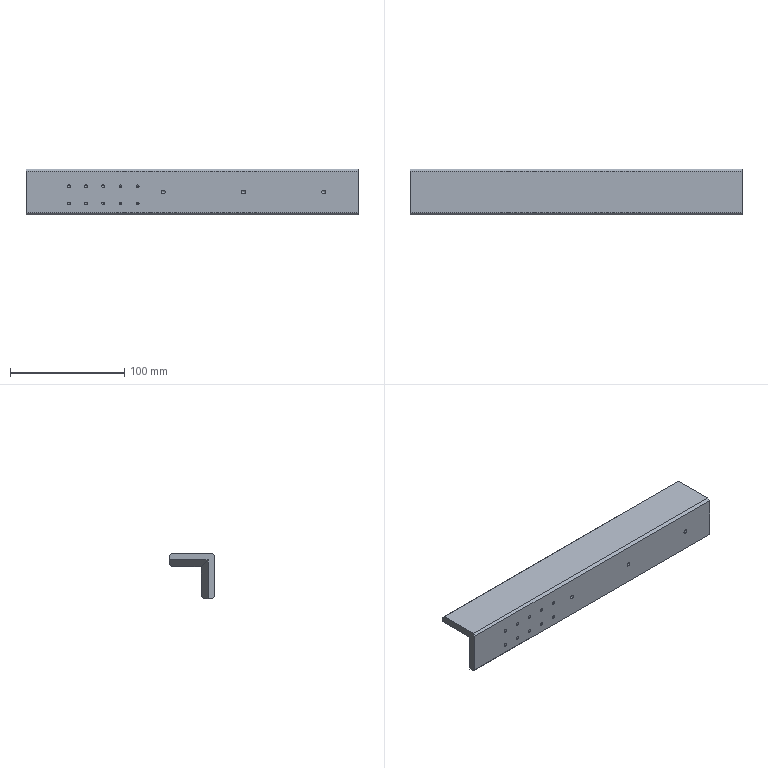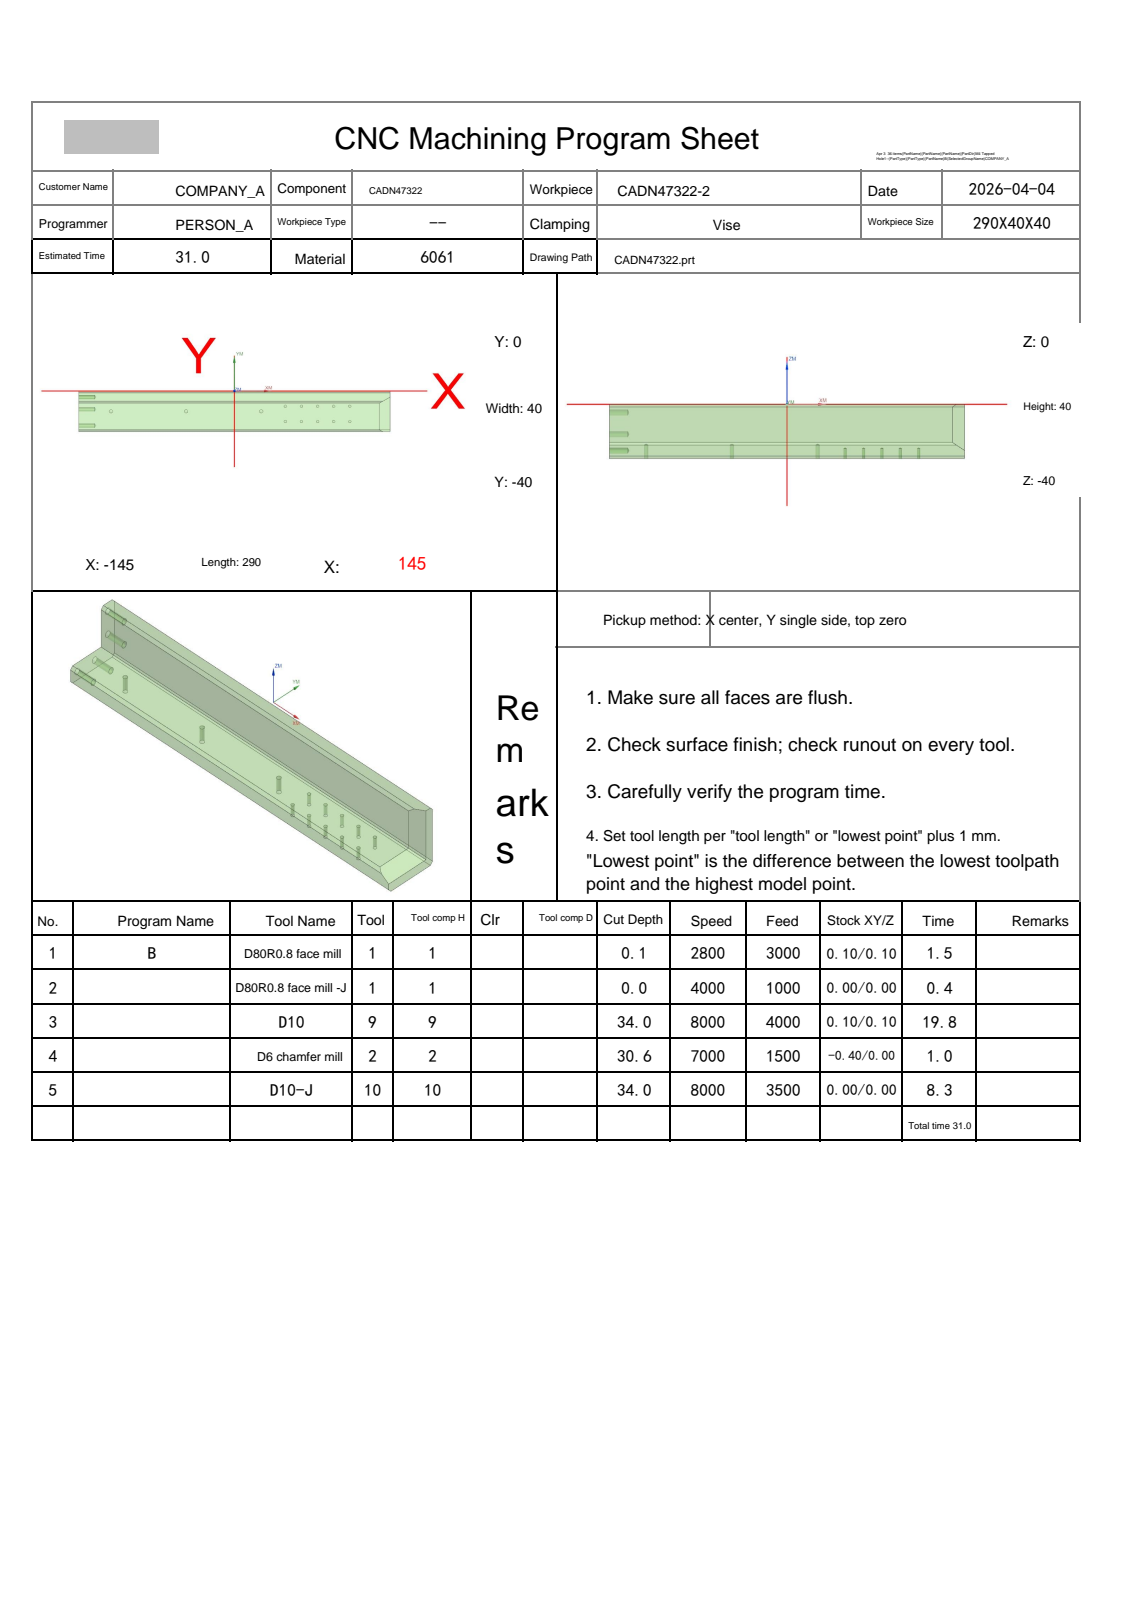NC program | NX | posted by the shop | part box 290 x 40 x 40 mm
Lines 3474 to 6219 of 6219, first 2289 of 2746 lines:
N4 T02 M06
(D6 chamfer mill  D=6. R=0. H=02 ce=0.00 di=0.00)
G00 G90 G54 X145.99 Y-1.208 M03 S6500
G43 H02 Z20.
M08
Z.13
G01 Z-1.2 F1500.
G03 X145.915 Y-1.548 I1.907 J-.601
G01 X145.905 Y-1.602
X145.928 Y-1.651
X145.966 Y-1.741
X146. Y-2.
Y-6.
X145.967 Y-6.255
X145.87 Y-6.493
X145.716 Y-6.698
X145.514 Y-6.857
X138.848 Y-10.857
X138.6 Y-10.964
X138.534 Y-10.973
X138.51 Y-10.969
X138.495 Y-10.989
X138.435 Y-11.027
X138.393 Y-11.083
Z.314
G00 Z10.
X-145.99 Y-10.792
Z.13
G01 Z-1.2
G03 X-145.915 Y-10.452 I-1.907 J.601
G01 X-145.905 Y-10.398
X-145.928 Y-10.349
X-145.966 Y-10.259
X-146. Y-10.
Y-2.
X-145.966 Y-1.741
X-145.928 Y-1.651
X-145.905 Y-1.602
X-145.915 Y-1.548
G03 X-145.99 Y-1.208 I-1.983 J-.261
G01 Z.13
G00 Z10.
X-145.916 Y-38.379
Z-25.199
G01 Z-29.199
X-145.966 Y-38.259
X-146. Y-38.
Y-15.123
X-146.008 Y-15.093
X-146.068 Y-15.007
Z-3.084
G00 Z20.
G00 G90 X-148.9 Y1.516 M03 S6500
Z20.
Z-1.2
G01 Z-2.7 F1000.
G03 X-147.763 Y.7 I1.137 J.384
G01 X147.763
G03 X148.9 Y1.516 I0.0 J1.2
G01 Z-1.2
G00 Z20.
X140.284 Y-13.378
Z-1.2
G01 Z-2.7
G03 X139.204 Y-12.7 I-1.08 J-.522
G01 X-147.763
G03 X-148.9 Y-13.516 I0.0 J-1.2
G01 Z-1.2
G00 Z20.
G00 G90 X142.5 Y-40.6 M03 S7000
Z20.
Z-28.1
G01 Z-30.6 F1000.
X135.
X-145.
X-152.5
Z-28.1
G00 Z20.
G91 G28 Z0.0
M05
M09
G91 G28 Z0.0
M01
N5 T10 M06
(D10-J  D=10. R=0. H=10 ce=0.40 di=0.00)
G00 G90 G54 X142. Y-40.999 M03 S7000
G43 H10 Z14.5
M08
Z-26.5
G01 Z-28. F1500.
G03 X140. Y-39. I-2. J-.001
G01 X-149.1
G02 X-150. Y-38.1 I0.0 J.9
G01 Y-35.68
G02 X-149. Y-34.68 I1. J0.0
G01 X139.1
G03 X140. Y-33.78 I0.0 J.9
G01 Y-31.36
G03 X139. Y-30.36 I-1. J0.0
G01 X-149.1
G02 X-150. Y-29.46 I0.0 J.9
G01 Y-27.04
G02 X-149. Y-26.04 I1. J0.0
G01 X139.1
G03 X140. Y-25.14 I0.0 J.9
G01 Y-22.72
G03 X139. Y-21.72 I-1. J0.0
G01 X-149.1
G02 X-150. Y-20.82 I0.0 J.9
G01 Y-18.4
G02 X-149. Y-17.4 I1. J0.0
G01 X140.
G02 X142. Y-19.399 I0.0 J-2.
G01 Z-26.5
G00 Z14.5
G00 G90 X149.655 Y-10.817 M03 S8000
Z9.5
Z-13.
G01 Z-14. F1000.
G41 D10
X149.533 Y-10.659
G03 X148.344 Y-10.074 I-1.189 J-.915
X147.572 Y-10.287 I0.0 J-1.5
G01 X137.572 Y-16.287
G02 X135. Y-17. I-2.572 J4.287
G01 X-145.
G03 X-146.49 Y-18.327 I0.0 J-1.5
G01 G40 X-146.513 Y-18.526
Z-13.
G00 Z9.5
X149.655 Y-10.817
Z-27.
G01 Z-28.
G41 D10
X149.533 Y-10.659
G03 X148.344 Y-10.074 I-1.189 J-.915
X147.572 Y-10.287 I0.0 J-1.5
G01 X137.572 Y-16.287
G02 X135. Y-17. I-2.572 J4.287
G01 X-145.
G03 X-146.49 Y-18.327 I0.0 J-1.5
G01 G40 X-146.513 Y-18.526
Z-27.
G00 Z9.5
G00 G90 X145.023 Y-17.66 M03 S7000
Z14.5
Z-27.508
G01 Z-28.008 F3500.
X140.023 Y-14.829
Y-39.163
X140.021 Y-39.21
X140.034 Y-39.218 Z-28.015
X140.036 Y-39.163
Y-14.821
X140.049 Y-14.813 Z-28.023
Y-39.163
X140.046 Y-39.226
X140.059 Y-39.233 Z-28.031
X140.061 Y-39.163
Y-14.806
X140.074 Y-14.798 Z-28.039
Y-39.163
X140.072 Y-39.241
X140.084 Y-39.249 Z-28.046
X140.087 Y-39.163
Y-14.79
X140.1 Y-14.783 Z-28.054
Y-39.163
X140.097 Y-39.257
X140.11 Y-39.265 Z-28.062
X140.113 Y-39.163
Y-14.775
X140.126 Y-14.767 Z-28.069
Y-39.163
X140.123 Y-39.272
X140.135 Y-39.28 Z-28.077
X140.139 Y-39.163
Y-14.759
X140.151 Y-14.752 Z-28.085
Y-39.163
X140.148 Y-39.288
X140.161 Y-39.296 Z-28.093
X140.164 Y-39.163
Y-14.744
X140.177 Y-14.736 Z-28.1
Y-39.163
X140.174 Y-39.304
X140.187 Y-39.311 Z-28.108
X140.19 Y-39.163
Y-14.729
X140.203 Y-14.721 Z-28.116
Y-39.163
X140.2 Y-39.319
X140.213 Y-39.327 Z-28.123
X140.216 Y-39.163
Y-14.713
X140.229 Y-14.705 Z-28.131
Y-39.163
X140.226 Y-39.335
X140.238 Y-39.343 Z-28.139
X140.242 Y-39.163
Y-14.698
X140.254 Y-14.69 Z-28.147
Y-39.163
X140.251 Y-39.35
X140.266 Y-39.358 Z-28.154
X140.267 Y-39.163
Y-14.682
X140.28 Y-14.675 Z-28.162
Y-39.163
X140.277 Y-39.366
X140.29 Y-39.374 Z-28.17
X140.293 Y-39.163
Y-14.667
X140.306 Y-14.659 Z-28.178
Y-39.163
X140.303 Y-39.382
X140.316 Y-39.389 Z-28.185
X140.319 Y-39.163
Y-14.651
X140.332 Y-14.644 Z-28.193
Y-39.163
X140.329 Y-39.397
X140.342 Y-39.405 Z-28.201
X140.344 Y-38.201
Y-14.636
X140.357 Y-14.628 Z-28.208
Y-38.208
X140.355 Y-39.413
X140.367 Y-39.421 Z-28.216
X140.37 Y-38.216
Y-14.621
X140.383 Y-14.613 Z-28.224
Y-38.224
X140.38 Y-39.428
X140.393 Y-39.436 Z-28.232
X140.396 Y-38.232
Y-14.605
X140.409 Y-14.597 Z-28.239
Y-38.239
X140.406 Y-39.444
X140.419 Y-39.452 Z-28.247
X140.422 Y-38.247
Y-14.59
X140.434 Y-14.582 Z-28.255
Y-38.255
X140.432 Y-39.459
X140.445 Y-39.467 Z-28.262
X140.447 Y-38.262
Y-14.574
X140.46 Y-14.567 Z-28.27
Y-38.27
X140.458 Y-39.475
X140.471 Y-39.483 Z-28.278
X140.473 Y-38.278
Y-14.559
X140.486 Y-14.551 Z-28.286
Y-38.286
X140.484 Y-39.491
X140.497 Y-39.498 Z-28.293
X140.499 Y-38.293
Y-14.543
X140.512 Y-14.536 Z-28.301
Y-38.301
X140.51 Y-39.506
X140.523 Y-39.514 Z-28.309
X140.524 Y-38.309
Y-14.528
X140.537 Y-14.52 Z-28.316
Y-38.316
X140.536 Y-39.522
X140.549 Y-39.53 Z-28.324
X140.55 Y-38.324
Y-14.512
X140.563 Y-14.505 Z-28.332
Y-38.332
X140.562 Y-39.537
X140.575 Y-39.545 Z-28.34
X140.576 Y-38.34
Y-14.497
X140.589 Y-14.489 Z-28.347
Y-38.347
X140.588 Y-39.553
X140.601 Y-39.561 Z-28.355
X140.602 Y-38.355
Y-14.482
X140.615 Y-14.474 Z-28.363
Y-38.363
X140.614 Y-39.569
X140.627 Y-39.576 Z-28.37
Y-38.37
Y-14.466
X140.64 Y-14.458 Z-28.378
Y-38.378
Y-39.584
X140.653 Y-39.592 Z-28.386
Y-38.386
Y-14.451
X140.666 Y-14.443 Z-28.394
Y-38.394
Y-39.6
X140.679 Y-39.607 Z-28.401
Y-38.401
Y-14.435
X140.692 Y-14.428 Z-28.409
Y-38.409
X140.691 Y-39.615
X140.704 Y-39.623 Z-28.417
X140.705 Y-38.417
Y-14.42
X140.717 Y-14.412 Z-28.424
Y-38.424
Y-39.631
X140.729 Y-39.638 Z-28.432
X140.73 Y-39.61
Y-14.404
X140.743 Y-14.397 Z-28.44
Y-39.61
X140.742 Y-39.646
X140.754 Y-39.654 Z-28.448
X140.756 Y-39.61
Y-14.389
X140.769 Y-14.381 Z-28.455
Y-39.61
X140.767 Y-39.661
X140.78 Y-39.669 Z-28.463
X140.782 Y-39.61
Y-14.374
X140.795 Y-14.366 Z-28.471
Y-39.61
X140.792 Y-39.677
X140.805 Y-39.685 Z-28.478
X140.807 Y-39.61
Y-14.358
X140.82 Y-14.35 Z-28.486
Y-39.61
X140.818 Y-39.692
X140.83 Y-39.7 Z-28.494
X140.833 Y-39.61
Y-14.343
X140.846 Y-14.335 Z-28.502
Y-39.61
X140.843 Y-39.708
X140.856 Y-39.715 Z-28.509
X140.859 Y-39.61
Y-14.327
X140.872 Y-14.32 Z-28.517
Y-39.61
X140.869 Y-39.723
X140.881 Y-39.731 Z-28.525
X140.885 Y-39.61
Y-14.312
X140.898 Y-14.304 Z-28.533
Y-39.61
X140.894 Y-39.738
X140.907 Y-39.746 Z-28.54
X140.91 Y-39.61
Y-14.296
X140.923 Y-14.289 Z-28.548
Y-39.61
X140.92 Y-39.754
X140.933 Y-39.761 Z-28.556
X140.936 Y-39.61
Y-14.281
X140.949 Y-14.273 Z-28.563
Y-39.61
X140.945 Y-39.769
X140.958 Y-39.777 Z-28.571
X140.962 Y-39.61
Y-14.266
X140.975 Y-14.258 Z-28.579
Y-39.61
X140.971 Y-39.785
X140.984 Y-39.792 Z-28.587
X140.988 Y-39.61
Y-14.25
X141. Y-14.242 Z-28.594
Y-39.61
X140.997 Y-39.8
X141.01 Y-39.808 Z-28.602
X141.013 Y-39.61
Y-14.235
X141.026 Y-14.227 Z-28.61
Y-39.61
X141.023 Y-39.815
X141.036 Y-39.823 Z-28.617
X141.039 Y-39.61
Y-14.219
X141.052 Y-14.212 Z-28.625
Y-39.61
X141.049 Y-39.831
X141.062 Y-39.838 Z-28.633
X141.065 Y-39.61
Y-14.204
X141.078 Y-14.196 Z-28.641
Y-39.61
X141.075 Y-39.846
X141.088 Y-39.854 Z-28.648
X141.09 Y-38.648
Y-14.188
X141.103 Y-14.181 Z-28.656
Y-38.656
X141.101 Y-39.862
X141.114 Y-39.869 Z-28.664
X141.116 Y-38.664
Y-14.173
X141.129 Y-14.165 Z-28.671
Y-38.671
X141.127 Y-39.877
X141.14 Y-39.885 Z-28.679
X141.142 Y-38.679
Y-14.157
X141.155 Y-14.15 Z-28.687
Y-38.687
X141.153 Y-39.892
X141.166 Y-39.9 Z-28.695
X141.168 Y-38.695
Y-14.142
X141.18 Y-14.134 Z-28.702
Y-38.702
X141.179 Y-39.908
X141.192 Y-39.915 Z-28.71
X141.193 Y-38.71
Y-14.127
X141.206 Y-14.119 Z-28.718
Y-38.718
X141.205 Y-39.923
X141.218 Y-39.931 Z-28.725
X141.219 Y-38.725
Y-14.111
X141.232 Y-14.103 Z-28.733
Y-38.733
X141.23 Y-39.939
X141.243 Y-39.946 Z-28.741
X141.245 Y-38.741
Y-14.096
X141.258 Y-14.088 Z-28.749
Y-38.749
X141.256 Y-39.954
X141.269 Y-39.962 Z-28.756
X141.271 Y-38.756
Y-14.08
X141.283 Y-14.073 Z-28.764
Y-38.764
X141.282 Y-39.969
X141.295 Y-39.977 Z-28.772
X141.296 Y-38.772
Y-14.065
X141.309 Y-14.057 Z-28.779
Y-38.779
X141.308 Y-39.985
X141.321 Y-39.992 Z-28.787
X141.322 Y-38.787
Y-14.049
X141.335 Y-14.042 Z-28.795
Y-38.795
X141.334 Y-40.
X141.347 Y-40.008 Z-28.803
X141.348 Y-38.803
Y-14.034
X141.361 Y-14.026 Z-28.81
Y-38.81
X141.36 Y-40.016
X141.373 Y-40.023 Z-28.818
Y-38.818
Y-14.019
X141.386 Y-14.011 Z-28.826
Y-38.826
Y-40.031
X141.399 Y-40.039 Z-28.833
Y-38.834
Y-14.003
X141.412 Y-13.995 Z-28.841
Y-38.841
Y-40.046
X141.425 Y-40.054 Z-28.849
Y-38.849
Y-13.988
X141.438 Y-13.98 Z-28.857
Y-38.857
Y-40.062
X141.45 Y-40.069 Z-28.864
X141.451 Y-38.864
Y-13.972
X141.463 Y-13.965 Z-28.872
Y-38.872
Y-40.077
X141.475 Y-40.085 Z-28.88
X141.476 Y-40.057
Y-13.957
X141.489 Y-13.949 Z-28.888
Y-40.057
X141.488 Y-40.092
X141.5 Y-40.1 Z-28.895
X141.502 Y-40.057
Y-13.941
X141.515 Y-13.934 Z-28.903
Y-40.057
X141.513 Y-40.108
X141.526 Y-40.116 Z-28.911
X141.528 Y-40.057
Y-13.926
X141.541 Y-13.918 Z-28.918
Y-40.057
X141.538 Y-40.123
X141.551 Y-40.131 Z-28.926
X141.553 Y-40.057
Y-13.911
X141.566 Y-13.903 Z-28.934
Y-40.057
X141.564 Y-40.139
X141.577 Y-40.146 Z-28.942
X141.579 Y-40.057
Y-13.895
X141.592 Y-13.887 Z-28.949
Y-40.057
X141.589 Y-40.154
X141.602 Y-40.162 Z-28.957
X141.605 Y-40.057
Y-13.88
X141.618 Y-13.872 Z-28.965
Y-40.057
X141.615 Y-40.169
X141.628 Y-40.177 Z-28.972
X141.631 Y-40.057
Y-13.864
X141.644 Y-13.857 Z-28.98
Y-40.057
X141.64 Y-40.185
X141.653 Y-40.192 Z-28.988
X141.656 Y-40.057
Y-13.849
X141.669 Y-13.841 Z-28.996
Y-40.057
X141.666 Y-40.2
X141.679 Y-40.208 Z-29.003
X141.682 Y-40.057
Y-13.833
X141.695 Y-13.826 Z-29.011
Y-40.057
X141.692 Y-40.215
X141.704 Y-40.223 Z-29.019
X141.708 Y-40.057
Y-13.818
X141.721 Y-13.81 Z-29.026
Y-40.057
X141.717 Y-40.231
X141.73 Y-40.238 Z-29.034
X141.734 Y-40.057
Y-13.802
X141.746 Y-13.795 Z-29.042
Y-40.057
X141.743 Y-40.246
X141.756 Y-40.253 Z-29.05
X141.759 Y-40.057
Y-13.787
X141.772 Y-13.779 Z-29.057
Y-40.057
X141.769 Y-40.261
X141.782 Y-40.269 Z-29.065
X141.785 Y-40.057
Y-13.772
X141.798 Y-13.764 Z-29.073
Y-40.057
X141.795 Y-40.276
X141.807 Y-40.284 Z-29.08
X141.811 Y-40.057
Y-13.756
X141.824 Y-13.748 Z-29.088
Y-40.057
X141.82 Y-40.292
X141.833 Y-40.299 Z-29.096
X141.836 Y-39.096
Y-13.741
X141.849 Y-13.733 Z-29.104
Y-39.104
X141.846 Y-40.307
X141.859 Y-40.315 Z-29.111
X141.862 Y-39.111
Y-13.725
X141.875 Y-13.718 Z-29.119
Y-39.119
X141.872 Y-40.322
X141.885 Y-40.33 Z-29.127
X141.888 Y-39.127
Y-13.71
X141.901 Y-13.702 Z-29.134
Y-39.134
X141.898 Y-40.338
X141.911 Y-40.345 Z-29.142
X141.914 Y-39.142
Y-13.694
X141.926 Y-13.687 Z-29.15
Y-39.15
X141.924 Y-40.353
X141.937 Y-40.361 Z-29.158
X141.939 Y-39.158
Y-13.679
X141.952 Y-13.671 Z-29.165
Y-39.165
X141.95 Y-40.368
X141.963 Y-40.376 Z-29.173
X141.965 Y-39.173
Y-13.664
X141.978 Y-13.656 Z-29.181
Y-39.181
X141.976 Y-40.384
X141.989 Y-40.391 Z-29.188
X141.991 Y-39.189
Y-13.648
X142.004 Y-13.64 Z-29.196
Y-39.196
X142.002 Y-40.399
X142.016 Y-40.407 Z-29.204
X142.017 Y-39.204
Y-13.633
X142.029 Y-13.625 Z-29.212
Y-39.212
Y-40.414
X142.042 Y-40.422 Z-29.219
Y-39.219
Y-13.617
X142.055 Y-13.61 Z-29.227
Y-39.227
Y-40.429
X142.067 Y-40.437 Z-29.235
X142.068 Y-39.235
Y-13.602
X142.081 Y-13.594 Z-29.243
Y-39.243
X142.08 Y-40.445
X142.093 Y-40.452 Z-29.25
X142.094 Y-39.25
Y-13.586
X142.107 Y-13.579 Z-29.258
Y-39.258
X142.106 Y-40.46
X142.119 Y-40.467 Z-29.266
Y-39.266
Y-13.571
X142.132 Y-13.563 Z-29.273
Y-39.273
Y-40.475
X142.145 Y-40.483 Z-29.281
Y-39.281
Y-13.556
X142.158 Y-13.548 Z-29.289
Y-39.289
Y-40.49
X142.171 Y-40.498 Z-29.297
Y-39.297
Y-13.54
X142.184 Y-13.532 Z-29.304
Y-39.304
Y-40.505
X142.196 Y-40.513 Z-29.312
X142.197 Y-39.312
Y-13.525
X142.209 Y-13.517 Z-29.32
Y-39.32
Y-40.521
X142.221 Y-40.528 Z-29.327
X142.222 Y-39.327
Y-13.509
X142.235 Y-13.501 Z-29.335
Y-40.505
X142.234 Y-40.536
X142.246 Y-40.543 Z-29.343
X142.248 Y-40.505
Y-13.494
X142.261 Y-13.486 Z-29.351
Y-40.505
X142.259 Y-40.551
X142.272 Y-40.558 Z-29.358
X142.274 Y-40.505
Y-13.478
X142.287 Y-13.471 Z-29.366
Y-40.505
X142.284 Y-40.566
X142.297 Y-40.574 Z-29.374
X142.3 Y-40.505
Y-13.463
X142.312 Y-13.455 Z-29.381
Y-40.505
X142.31 Y-40.581
X142.322 Y-40.589 Z-29.389
X142.325 Y-40.505
Y-13.447
X142.338 Y-13.44 Z-29.397
Y-40.505
X142.335 Y-40.596
X142.348 Y-40.604 Z-29.405
X142.351 Y-40.505
Y-13.432
X142.364 Y-13.424 Z-29.412
Y-40.505
X142.361 Y-40.612
X142.374 Y-40.619 Z-29.42
X142.377 Y-40.505
Y-13.417
X142.39 Y-13.409 Z-29.428
Y-40.505
X142.386 Y-40.627
X142.399 Y-40.634 Z-29.435
X142.402 Y-40.505
Y-13.401
X142.415 Y-13.393 Z-29.443
Y-40.505
X142.412 Y-40.642
X142.425 Y-40.65 Z-29.451
X142.428 Y-40.505
Y-13.386
X142.441 Y-13.378 Z-29.459
Y-40.505
X142.438 Y-40.657
X142.451 Y-40.665 Z-29.466
X142.454 Y-40.505
Y-13.37
X142.467 Y-13.363 Z-29.474
Y-40.505
X142.464 Y-40.672
X142.479 Y-40.68 Z-29.482
X142.48 Y-39.482
Y-13.355
X142.492 Y-13.347 Z-29.489
Y-40.505
X142.49 Y-40.688
X142.502 Y-40.695 Z-29.497
X142.505 Y-40.505
Y-13.339
X142.518 Y-13.332 Z-29.505
Y-40.505
X142.515 Y-40.703
X142.528 Y-40.71 Z-29.513
X142.531 Y-40.505
Y-13.324
X142.544 Y-13.316 Z-29.52
Y-40.505
X142.541 Y-40.718
X142.554 Y-40.726 Z-29.528
X142.557 Y-40.505
Y-13.309
X142.57 Y-13.301 Z-29.536
Y-40.505
X142.567 Y-40.733
X142.58 Y-40.741 Z-29.543
X142.582 Y-40.505
Y-13.293
X142.595 Y-13.285 Z-29.551
Y-39.551
X142.592 Y-40.749
X142.605 Y-40.756 Z-29.559
X142.608 Y-39.559
Y-13.278
X142.621 Y-13.27 Z-29.567
Y-39.567
X142.618 Y-40.764
X142.631 Y-40.771 Z-29.574
X142.634 Y-39.574
Y-13.262
X142.647 Y-13.255 Z-29.582
Y-39.582
X142.644 Y-40.779
X142.657 Y-40.787 Z-29.59
X142.66 Y-39.59
Y-13.247
X142.673 Y-13.239 Z-29.598
Y-39.598
X142.67 Y-40.794
X142.683 Y-40.802 Z-29.605
X142.685 Y-39.605
Y-13.231
X142.698 Y-13.224 Z-29.613
Y-39.613
X142.696 Y-40.809
X142.709 Y-40.817 Z-29.621
X142.711 Y-39.621
Y-13.216
X142.724 Y-13.208 Z-29.628
Y-39.628
X142.722 Y-40.825
X142.735 Y-40.832 Z-29.636
X142.737 Y-39.636
Y-13.201
X142.75 Y-13.193 Z-29.644
Y-39.644
X142.748 Y-40.84
X142.761 Y-40.847 Z-29.652
X142.763 Y-39.652
Y-13.185
X142.775 Y-13.177 Z-29.659
Y-39.659
X142.774 Y-40.855
X142.787 Y-40.863 Z-29.667
X142.788 Y-39.667
Y-13.17
X142.801 Y-13.162 Z-29.675
Y-39.675
X142.8 Y-40.87
X142.813 Y-40.878 Z-29.682
X142.814 Y-39.682
Y-13.154
X142.827 Y-13.146 Z-29.69
Y-39.69
X142.826 Y-40.885
X142.839 Y-40.893 Z-29.698
X142.84 Y-39.698
Y-13.139
X142.853 Y-13.131 Z-29.706
Y-39.706
X142.852 Y-40.901
X142.865 Y-40.908 Z-29.713
Y-39.713
Y-13.123
X142.878 Y-13.116 Z-29.721
Y-39.721
Y-40.916
X142.891 Y-40.923 Z-29.729
Y-39.729
Y-13.108
X142.904 Y-13.1 Z-29.736
Y-39.736
Y-40.931
X142.917 Y-40.939 Z-29.744
Y-39.744
Y-13.092
X142.93 Y-13.085 Z-29.752
Y-39.752
Y-40.946
X142.943 Y-40.953 Z-29.76
Y-39.76
Y-13.077
X142.955 Y-13.069 Z-29.767
Y-39.767
Y-40.956
X142.968 Y-40.959 Z-29.775
Y-39.775
Y-13.062
X142.981 Y-13.054 Z-29.783
Y-39.783
Y-40.963
X142.993 Y-40.966 Z-29.79
X142.994 Y-39.79
Y-13.046
X143.007 Y-13.038 Z-29.798
Y-39.798
X143.006 Y-40.969
X143.019 Y-40.973 Z-29.806
X143.02 Y-39.806
Y-13.031
X143.033 Y-13.023 Z-29.814
Y-39.814
X143.032 Y-40.976
X143.044 Y-40.979 Z-29.821
X143.046 Y-40.952
Y-13.015
X143.058 Y-13.008 Z-29.829
Y-40.952
X143.057 Y-40.983
X143.07 Y-40.986 Z-29.837
X143.071 Y-40.952
Y-13.
X143.084 Y-12.992 Z-29.844
Y-40.952
X143.083 Y-40.989
X143.095 Y-40.993 Z-29.852
X143.097 Y-40.952
Y-12.984
X143.11 Y-12.977 Z-29.86
Y-40.952
X143.108 Y-40.996
X143.121 Y-41. Z-29.868
X143.123 Y-40.952
Y-12.969
X143.136 Y-12.961 Z-29.875
Y-40.952
X143.134 Y-41.003
X143.147 Y-41.006 Z-29.883
X143.148 Y-40.952
Y-12.954
X143.161 Y-12.946 Z-29.891
Y-40.952
X143.159 Y-41.01
X143.172 Y-41.013 Z-29.898
X143.174 Y-40.952
Y-12.938
X143.187 Y-12.93 Z-29.906
Y-40.952
X143.185 Y-41.016
X143.198 Y-41.02 Z-29.914
X143.2 Y-40.952
Y-12.923
X143.213 Y-12.915 Z-29.922
Y-40.952
X143.21 Y-41.023
X143.223 Y-41.026 Z-29.929
X143.226 Y-40.952
Y-12.907
X143.238 Y-12.9 Z-29.937
Y-40.952
X143.236 Y-41.03
X143.249 Y-41.033 Z-29.945
X143.251 Y-40.952
Y-12.892
X143.264 Y-12.884 Z-29.953
Y-40.952
X143.262 Y-41.036
X143.271 Y-41.039 Z-29.956
X143.274 Y-41.04 Z-29.96
X143.277 Y-40.952
Y-12.876
X143.29 Y-12.869 Z-29.968
Y-40.952
X143.287 Y-41.043
X143.296 Y-41.045 Z-29.972
X143.3 Y-41.046 Z-29.976
X143.303 Y-40.952
Y-12.861
X143.316 Y-12.853 Z-29.983
Y-40.952
X143.313 Y-41.05
X143.322 Y-41.052 Z-29.987
X143.326 Y-41.053 Z-29.991
X143.328 Y-40.952
Y-12.846
X143.341 Y-12.838 Z-29.999
Y-40.952
X143.339 Y-41.056
X143.348 Y-41.059 Z-30.003
X143.351 Y-41.06 Z-30.007
X143.354 Y-40.952
Y-12.83
X143.367 Y-12.822 Z-30.014
Y-40.952
X143.366 Y-41.062
X143.374 Z-30.018
X143.377 Z-30.022
X143.38 Y-40.952
Y-12.815
X143.393 Y-12.807 Z-30.03
Y-40.952
X143.39 Y-41.063
X143.399 Z-30.034
X143.403 Z-30.037
X143.406 Y-40.952
Y-12.799
X143.419 Y-12.791 Z-30.045
Y-40.952
X143.416 Y-41.063
X143.425 Z-30.049
X143.429 Z-30.053
X143.431 Y-40.952
Y-12.784
X143.444 Y-12.776 Z-30.061
Y-40.952
X143.441 Y-41.063
X143.451 Z-30.064
X143.454 Z-30.068
X143.457 Y-40.952
Y-12.768
X143.47 Y-12.761 Z-30.076
Y-40.952
X143.467 Y-41.063
X143.476 Z-30.08
X143.48 Z-30.084
X143.483 Y-40.952
Y-12.753
X143.496 Y-12.745 Z-30.091
Y-40.952
X143.493 Y-41.063
X143.502 Y-41.064 Z-30.095
X143.506 Z-30.099
X143.509 Y-40.952
Y-12.737
X143.521 Y-12.73 Z-30.107
Y-40.952
X143.519 Y-41.064
X143.528 Z-30.111
X143.531 Z-30.115
X143.534 Y-40.952
Y-12.722
X143.547 Y-12.714 Z-30.122
Y-40.952
X143.544 Y-41.064
X143.554 Z-30.126
X143.557 Z-30.13
X143.56 Y-40.952
Y-12.707
X143.573 Y-12.699 Z-30.138
Y-40.952
X143.57 Y-41.064
X143.579 Z-30.142
X143.583 Z-30.145
X143.586 Y-40.952
Y-12.691
X143.599 Y-12.683 Z-30.153
Y-40.952
X143.596 Y-41.064
X143.605 Z-30.157
X143.609 Z-30.161
X143.611 Y-40.952
Y-12.676
X143.624 Y-12.668 Z-30.169
Y-40.952
X143.622 Y-41.065
X143.631 Z-30.172
X143.634 Z-30.176
X143.637 Y-40.952
Y-12.66
X143.65 Y-12.653 Z-30.184
Y-40.952
X143.647 Y-41.065
X143.656 Z-30.188
X143.66 Z-30.192
X143.663 Y-40.952
Y-12.645
X143.676 Y-12.637 Z-30.199
Y-40.952
X143.673 Y-41.065
X143.682 Z-30.203
X143.686 Z-30.207
X143.689 Y-40.952
Y-12.629
X143.702 Y-12.622 Z-30.215
Y-40.952
X143.699 Y-41.065
X143.708 Z-30.219
X143.712 Z-30.223
X143.714 Y-40.952
Y-12.614
X143.727 Y-12.606 Z-30.23
Y-40.952
X143.724 Y-41.065
X143.734 Z-30.234
X143.737 Y-41.066 Z-30.238
X143.74 Y-40.952
Y-12.599
X143.753 Y-12.591 Z-30.246
Y-40.952
X143.75 Y-41.066
X143.759 Z-30.25
X143.763 Z-30.253
X143.766 Y-40.952
Y-12.583
X143.779 Y-12.575 Z-30.261
Y-40.952
X143.776 Y-41.066
X143.785 Z-30.265
X143.789 Z-30.269
X143.792 Y-40.952
Y-12.568
X143.804 Y-12.56 Z-30.277
Y-40.952
X143.802 Y-41.066
X143.811 Z-30.281
X143.815 Z-30.284
X143.817 Y-40.952
Y-12.552
X143.83 Y-12.545 Z-30.292
Y-40.952
X143.827 Y-41.066
X143.837 Z-30.296
X143.84 Z-30.3
X143.843 Y-40.952
Y-12.537
X143.856 Y-12.529 Z-30.308
Y-40.952
X143.853 Y-41.066
X143.862 Y-41.067 Z-30.311
X143.866 Z-30.315
X143.869 Y-40.952
Y-12.521
X143.882 Y-12.514 Z-30.323
Y-40.952
X143.879 Y-41.067
X143.888 Z-30.327
X143.892 Z-30.331
X143.894 Y-40.952
Y-12.506
X143.907 Y-12.498 Z-30.338
Y-40.952
X143.904 Y-41.067
X143.914 Z-30.342
X143.917 Z-30.346
X143.92 Y-40.952
Y-12.491
X143.933 Y-12.483 Z-30.354
Y-40.952
X143.93 Y-41.067
X143.939 Z-30.358
X143.943 Z-30.362
X143.946 Y-40.952
Y-12.475
X143.959 Y-12.467 Z-30.369
Y-40.952
X143.956 Y-41.067
X143.965 Z-30.373
X143.969 Z-30.377
X143.972 Y-40.952
Y-12.46
X143.984 Y-12.452 Z-30.385
Y-40.952
X143.982 Y-41.068
X143.991 Z-30.389
X143.995 Z-30.392
X143.997 Y-40.952
Y-12.444
X144.01 Y-12.436 Z-30.4
Y-40.952
X144.007 Y-41.068
X144.017 Z-30.404
X144.02 Z-30.408
X144.023 Y-40.952
Y-12.429
X144.036 Y-12.421 Z-30.416
Y-40.952
X144.033 Y-41.068
X144.042 Z-30.419
X144.046 Z-30.423
X144.049 Y-40.952
Y-12.413
X144.062 Y-12.406 Z-30.431
Y-40.952
X144.059 Y-41.068
X144.068 Z-30.435
X144.072 Z-30.439
X144.075 Y-40.952
Y-12.398
X144.087 Y-12.39 Z-30.446
Y-40.952
X144.085 Y-41.068
X144.094 Z-30.45
X144.097 Z-30.454
X144.1 Y-40.952
Y-12.382
X144.113 Y-12.375 Z-30.462
Y-40.952
X144.11 Y-41.069
X144.12 Z-30.466
X144.123 Z-30.47
X144.126 Y-40.952
Y-12.367
X144.139 Y-12.359 Z-30.477
Y-40.952
X144.136 Y-41.069
X144.145 Z-30.481
X144.149 Z-30.485
X144.152 Y-40.952
Y-12.352
X144.165 Y-12.344 Z-30.493
Y-40.952
X144.162 Y-41.069
X144.171 Z-30.497
X144.175 Z-30.5
X144.177 Y-40.952
Y-12.336
X144.19 Y-12.328 Z-30.508
Y-40.952
X144.187 Y-41.069
X144.197 Z-30.512
X144.2 Z-30.516
X144.203 Y-40.952
Y-12.321
X144.216 Y-12.313 Z-30.524
Y-40.952
X144.213 Y-41.069
X144.222 Y-41.07 Z-30.527
X144.226 Z-30.531
X144.229 Y-40.952
Y-12.305
X144.242 Y-12.298 Z-30.539
Y-40.952
X144.239 Y-41.07
X144.248 Z-30.543
X144.253 Z-30.547
X144.255 Y-40.952
Y-12.29
X144.267 Y-12.282 Z-30.554
Y-40.952
X144.265 Y-41.07
X144.274 Z-30.558
X144.277 Z-30.562
X144.28 Y-40.952
Y-12.274
X144.293 Y-12.267 Z-30.57
Y-40.952
X144.29 Y-41.07
X144.3 Z-30.574
X144.303 Z-30.578
X144.306 Y-40.952
Y-12.259
X144.319 Y-12.251 Z-30.585
Y-40.952
X144.316 Y-41.07
X144.325 Z-30.589
X144.329 Z-30.593
X144.332 Y-40.952
Y-12.244
X144.345 Y-12.236 Z-30.601
Y-40.952
X144.342 Y-41.07
X144.351 Y-41.071 Z-30.605
X144.355 Z-30.608
X144.357 Y-40.952
Y-12.228
X144.37 Y-12.22 Z-30.616
Y-40.952
X144.367 Y-41.071
X144.377 Z-30.62
X144.38 Z-30.624
X144.383 Y-40.952
Y-12.213
X144.396 Y-12.205 Z-30.632
Y-40.952
X144.393 Y-41.071
X144.403 Z-30.636
X144.406 Z-30.639
X144.409 Y-40.952
Y-12.197
X144.422 Y-12.19 Z-30.647
Y-40.952
X144.419 Y-41.071
X144.428 Z-30.651
X144.432 Z-30.655
X144.435 Y-40.952
Y-12.182
X144.448 Y-12.174 Z-30.663
Y-40.952
X144.445 Y-41.071
X144.454 Z-30.666
X144.458 Z-30.67
X144.46 Y-40.952
Y-12.166
X144.473 Y-12.159 Z-30.678
Y-40.952
X144.47 Y-41.072
X144.48 Z-30.682
X144.483 Z-30.686
X144.486 Y-40.952
Y-12.151
X144.499 Y-12.143 Z-30.693
Y-40.952
X144.496 Y-41.072
X144.505 Z-30.697
X144.509 Z-30.701
X144.512 Y-40.952
Y-12.136
X144.525 Y-12.128 Z-30.709
Y-40.952
X144.522 Y-41.072
X144.531 Z-30.713
X144.535 Z-30.717
X144.538 Y-40.952
Y-12.12
X144.55 Y-12.112 Z-30.724
Y-40.952
X144.548 Y-41.072
X144.557 Z-30.728
X144.56 Z-30.732
X144.563 Y-40.952
Y-12.105
X144.576 Y-12.097 Z-30.74
Y-40.952
X144.573 Y-41.072
X144.583 Z-30.744
X144.586 Z-30.747
X144.589 Y-40.952
Y-12.089
X144.602 Y-12.081 Z-30.755
Y-40.952
X144.599 Y-41.073
X144.608 Z-30.759
X144.612 Z-30.763
X144.615 Y-40.952
Y-12.074
X144.628 Y-12.066 Z-30.771
Y-40.952
X144.625 Y-41.073
X144.634 Z-30.774
X144.638 Z-30.778
X144.64 Y-40.952
Y-12.058
X144.653 Y-12.051 Z-30.786
Y-40.952
X144.65 Y-41.073
X144.66 Z-30.79
X144.663 Z-30.794
X144.666 Y-40.952
Y-12.043
X144.679 Y-12.035 Z-30.801
Y-40.952
X144.676 Y-41.073
X144.685 Z-30.805
X144.689 Z-30.809
X144.692 Y-40.952
Y-12.027
X144.705 Y-12.02 Z-30.817
Y-40.952
X144.702 Y-41.073
X144.711 Z-30.821
X144.715 Z-30.825
X144.718 Y-40.952
Y-12.012
X144.73 Y-12.004 Z-30.832
Y-40.952
X144.728 Y-41.074
X144.737 Z-30.836
X144.74 Z-30.84
X144.743 Y-40.952
Y-11.997
X144.756 Y-11.989 Z-30.848
Y-40.952
X144.753 Y-41.074
X144.763 Z-30.852
X144.766 Z-30.855
X144.769 Y-40.952
Y-11.981
X144.782 Y-11.973 Z-30.863
Y-40.952
X144.779 Y-41.074
X144.788 Z-30.867
X144.792 Z-30.871
X144.795 Y-40.952
Y-11.966
X144.808 Y-11.958 Z-30.879
Y-40.952
X144.805 Y-41.074
X144.814 Z-30.882
X144.818 Z-30.886
X144.821 Y-40.952
Y-11.95
X144.833 Y-11.943 Z-30.894
Y-40.952
X144.831 Y-41.074
X144.84 Z-30.898
X144.843 Z-30.902
X144.846 Y-40.952
Y-11.935
X144.859 Y-11.927 Z-30.909
Y-40.952
X144.856 Y-41.075
X144.866 Z-30.913
X144.869 Z-30.917
X144.872 Y-40.952
Y-11.919
X144.885 Y-11.912 Z-30.925
Y-40.952
X144.882 Y-41.075
X144.891 Z-30.929
X144.895 Z-30.933
X144.898 Y-40.952
Y-11.904
X144.911 Y-11.896 Z-30.94
Y-40.952
X144.908 Y-41.075
X144.917 Z-30.944
X144.921 Z-30.948
X144.923 Y-40.952
Y-11.889
X144.936 Y-11.881 Z-30.956
Y-40.952
X144.933 Y-41.075
X144.943 Z-30.96
X144.946 Z-30.963
X144.949 Y-40.952
Y-11.873
X144.962 Y-11.865 Z-30.971
Y-40.952
X144.959 Y-41.075
X144.968 Z-30.975
X144.972 Z-30.979
X144.975 Y-40.952
Y-11.858
X144.988 Y-11.85 Z-30.987
Y-40.952
X144.985 Y-41.075
X144.994 Y-41.076 Z-30.991
X144.998 Z-30.994
X145.001 Y-40.952
Y-11.842
X145.013 Y-11.835 Z-31.002
Y-40.952
X145.011 Y-41.076
X145.02 Z-31.006
X145.023 Z-31.01
X145.026 Y-40.952
Y-11.827
X145.039 Y-11.819 Z-31.018
Y-40.952
X145.036 Y-41.076
X145.046 Z-31.021
X145.049 Z-31.025
X145.052 Y-40.952
Y-11.811
X145.065 Y-11.804 Z-31.033
Y-40.952
X145.062 Y-41.076
X145.071 Z-31.037
X145.075 Z-31.041
X145.078 Y-40.952
Y-11.796
X145.091 Y-11.788 Z-31.048
Y-40.952
X145.088 Y-41.076
X145.097 Z-31.052
X145.101 Z-31.056
X145.104 Y-40.952
Y-11.781
X145.116 Y-11.773 Z-31.064
Y-40.952
X145.113 Y-41.076
X145.123 Z-31.068
X145.126 Y-41.077 Z-31.072
X145.129 Y-40.952
Y-11.765
X145.142 Y-11.757 Z-31.079
Y-40.952
X145.14 Y-41.077
X145.149 Z-31.083
X145.152 Z-31.087
X145.155 Y-40.952
Y-11.75
X145.168 Y-11.742 Z-31.095
Y-40.952
X145.165 Y-41.077
X145.174 Z-31.099
X145.178 Z-31.102
X145.181 Y-40.952
Y-11.734
X145.194 Y-11.726 Z-31.11
Y-40.952
X145.191 Y-41.077
X145.2 Z-31.114
X145.204 Z-31.118
X145.206 Y-40.952
Y-11.719
X145.219 Y-11.711 Z-31.126
Y-40.952
X145.216 Y-41.077
X145.226 Z-31.129
X145.229 Z-31.133
X145.232 Y-40.952
Y-11.703
X145.245 Y-11.696 Z-31.141
Y-40.952
X145.242 Y-41.077
X145.251 Z-31.145
X145.255 Z-31.149
X145.258 Y-40.952
Y-11.688
X145.271 Y-11.68 Z-31.156
Y-40.952
X145.268 Y-41.077
X145.277 Z-31.16
X145.281 Z-31.164
X145.284 Y-40.952
Y-11.672
X145.296 Y-11.665 Z-31.172
Y-40.952
X145.294 Y-41.077
X145.303 Z-31.176
X145.306 Z-31.18
X145.309 Y-40.952
Y-11.657
X145.322 Y-11.649 Z-31.187
Y-40.952
X145.319 Y-41.077
X145.329 Z-31.191
X145.332 Z-31.195
X145.335 Y-40.952
Y-11.642
X145.348 Y-11.634 Z-31.203
Y-40.952
X145.345 Y-41.078
X145.354 Z-31.207
X145.358 Z-31.21
X145.361 Y-40.952
Y-11.626
X145.374 Y-11.618 Z-31.218
Y-40.952
X145.371 Y-41.078
X145.38 Z-31.222
X145.384 Z-31.226
X145.386 Y-40.952
Y-11.611
X145.399 Y-11.603 Z-31.234
Y-40.952
X145.396 Y-41.078
X145.406 Z-31.237
X145.409 Z-31.241
X145.412 Y-40.952
Y-11.595
X145.425 Y-11.588 Z-31.249
Y-40.952
X145.422 Y-41.078
X145.432 Z-31.253
X145.435 Z-31.257
X145.438 Y-40.952
Y-11.58
X145.451 Y-11.572 Z-31.264
Y-40.952
X145.448 Y-41.078
X145.457 Z-31.268
X145.461 Z-31.272
X145.464 Y-40.952
Y-11.564
X145.477 Y-11.557 Z-31.28
Y-40.952
X145.474 Y-41.078
X145.483 Z-31.284
X145.486 Z-31.288
X145.489 Y-40.952
Y-11.549
X145.502 Y-11.541 Z-31.295
Y-40.952
X145.499 Y-41.078
X145.509 Z-31.299
X145.512 Z-31.303
X145.515 Y-40.952
Y-11.534
X145.528 Y-11.526 Z-31.311
Y-40.952
X145.525 Y-41.078
X145.534 Z-31.315
X145.538 Z-31.318
X145.541 Y-40.952
Y-11.518
X145.554 Y-11.51 Z-31.326
Y-40.952
X145.551 Y-41.078
X145.56 Z-31.33
X145.564 Z-31.334
X145.567 Y-40.952
Y-11.503
X145.579 Y-11.495 Z-31.342
Y-40.
Y-41.079
X145.589 Z-31.349
X145.592 Y-40.952
Y-11.487
X145.605 Y-11.48 Z-31.357
Y-40.952
X145.602 Y-41.079
X145.612 Z-31.361
X145.615 Z-31.365
X145.618 Y-40.952
Y-11.472
X145.631 Y-11.464 Z-31.373
Y-40.952
X145.628 Y-41.079
X145.637 Z-31.376
X145.641 Z-31.38
X145.644 Y-40.952
Y-11.456
X145.657 Y-11.449 Z-31.388
Y-40.952
X145.654 Y-41.079
X145.663 Z-31.392
X145.667 Z-31.396
X145.669 Y-40.952
Y-11.441
X145.682 Y-11.433 Z-31.403
Y-40.952
X145.679 Y-41.079
X145.689 Z-31.407
X145.692 Z-31.411
X145.695 Y-40.952
Y-11.426
X145.708 Y-11.418 Z-31.419
Y-40.952
X145.705 Y-41.079
X145.714 Z-31.423
X145.718 Z-31.427
X145.721 Y-40.952
Y-11.41
X145.734 Y-11.402 Z-31.434
Y-40.952
X145.731 Y-41.079
X145.74 Z-31.438
X145.744 Z-31.442
X145.747 Y-40.952
Y-11.395
X145.759 Y-11.387 Z-31.45
Y-40.952
X145.757 Y-41.079
X145.766 Z-31.454
X145.769 Z-31.457
X145.772 Y-40.952
Y-11.379
X145.785 Y-11.371 Z-31.465
Y-40.952
X145.782 Y-41.079
X145.792 Z-31.469
X145.795 Y-41.08 Z-31.473
X145.798 Y-40.952
Y-11.364
X145.811 Y-11.356 Z-31.481
Y-40.952
X145.808 Y-41.08
X145.817 Z-31.484
X145.821 Z-31.488
X145.824 Y-40.952
Y-11.348
X145.837 Y-11.341 Z-31.496
Y-40.952
X145.834 Y-41.08
X145.843 Z-31.5
X145.847 Z-31.504
X145.85 Y-40.952
Y-11.333
X145.862 Y-11.325 Z-31.511
Y-40.952
X145.859 Y-41.08
X145.869 Z-31.515
X145.872 Z-31.519
X145.875 Y-40.952
Y-11.317
X145.888 Y-11.31 Z-31.527
Y-40.952
X145.885 Y-41.08
X145.895 Z-31.531
X145.898 Z-31.535
X145.901 Y-40.952
Y-11.302
X145.914 Y-11.294 Z-31.542
Y-40.952
X145.911 Y-41.08
X145.92 Z-31.546
X145.924 Z-31.55
X145.927 Y-40.952
Y-11.287
X145.94 Y-11.279 Z-31.558
Y-40.952
X145.937 Y-41.08
X145.946 Z-31.562
X145.95 Z-31.565
X145.952 Y-40.952
Y-11.271
X145.965 Y-11.263 Z-31.573
Y-40.952
X145.962 Y-41.08
X145.972 Z-31.577
X145.975 Z-31.581
X145.978 Y-40.952
Y-11.256
X145.991 Y-11.248 Z-31.589
Y-40.952
X145.988 Y-41.08
X145.997 Z-31.592
X146.001 Z-31.596
X146.004 Y-40.952
Y-11.24
X146.017 Y-11.233 Z-31.604
Y-40.952
X146.014 Y-41.08
X146.023 Y-41.081 Z-31.608
X146.027 Z-31.612
X146.03 Y-40.952
Y-11.225
X146.042 Y-11.217 Z-31.619
Y-40.952
X146.04 Y-41.081
X146.049 Z-31.623
X146.052 Z-31.627
X146.055 Y-40.952
Y-11.209
X146.068 Y-11.202 Z-31.635
Y-40.952
X146.065 Y-41.081
X146.075 Z-31.639
X146.078 Z-31.643
X146.081 Y-40.952
Y-11.194
X146.094 Y-11.186 Z-31.65
Y-40.952
X146.091 Y-41.081
X146.1 Z-31.654
X146.104 Z-31.658
X146.107 Y-40.952
Y-11.179
X146.12 Y-11.171 Z-31.666
Y-40.952
X146.117 Y-41.081
X146.126 Z-31.67
X146.13 Z-31.674
X146.133 Y-40.952
Y-11.163
X146.145 Y-11.155 Z-31.681
Y-40.952
X146.142 Y-41.081
X146.152 Z-31.685
X146.155 Z-31.689
X146.158 Y-40.952
Y-11.148
X146.171 Y-11.14 Z-31.697
Y-40.952
X146.168 Y-41.081
X146.178 Z-31.701
X146.181 Z-31.704
X146.184 Y-40.952
Y-11.132
X146.197 Y-11.125 Z-31.712
Y-40.952
X146.194 Y-41.081
X146.203 Z-31.716
X146.207 Z-31.72
X146.21 Y-40.952
Y-11.117
X146.223 Y-11.109 Z-31.728
Y-40.952
X146.22 Y-41.081
X146.229 Z-31.731
X146.232 Z-31.735
X146.235 Y-40.952
Y-11.101
X146.248 Y-11.094 Z-31.743
Y-40.952
X146.245 Y-41.081
X146.255 Y-41.082 Z-31.747
X146.258 Z-31.751
X146.261 Y-40.952
Y-11.086
X146.274 Y-11.078 Z-31.758
Y-40.952
X146.271 Y-41.082
X146.28 Z-31.762
X146.284 Z-31.766
X146.287 Y-40.952
Y-11.071
X146.3 Y-11.063 Z-31.774
Y-40.952
X146.297 Y-41.082
X146.306 Z-31.778
X146.31 Z-31.782
X146.313 Y-40.952
Y-11.055
X146.325 Y-11.047 Z-31.789
Y-40.952
X146.323 Y-41.082
X146.332 Z-31.793
X146.335 Z-31.797
X146.338 Y-40.952
Y-11.04
X146.351 Y-11.032 Z-31.805
Y-40.952
X146.348 Y-41.082
X146.358 Z-31.809
X146.361 Z-31.812
X146.364 Y-40.952
Y-11.024
X146.377 Y-11.016 Z-31.82
Y-40.952
X146.374 Y-41.082
X146.383 Z-31.824
X146.387 Z-31.828
X146.39 Y-40.952
Y-11.009
X146.403 Y-11.001 Z-31.836
Y-40.952
X146.4 Y-41.082
X146.409 Z-31.839
X146.413 Z-31.843
X146.415 Y-40.952
Y-10.993
X146.428 Y-10.986 Z-31.851
Y-40.952
X146.425 Y-41.082
X146.435 Z-31.855
X146.438 Z-31.859
X146.441 Y-40.952
Y-10.978
X146.454 Y-10.97 Z-31.866
Y-40.952
X146.451 Y-41.082
X146.466 Y-41.083 Z-31.874
X146.467 Y-40.952
Y-10.962
X146.48 Y-10.955 Z-31.882
Y-40.952
X146.477 Y-41.082
X146.486 Z-31.886
X146.49 Y-41.083 Z-31.89
X146.493 Y-40.952
Y-10.947
X146.506 Y-10.939 Z-31.897
Y-40.952
X146.503 Y-41.083
X146.512 Z-31.901
X146.515 Z-31.905
X146.518 Y-40.952
Y-10.932
X146.531 Y-10.924 Z-31.913
Y-40.952
X146.528 Y-41.083
X146.538 Z-31.917
X146.541 Z-31.92
X146.544 Y-40.952
Y-10.916
X146.557 Y-10.908 Z-31.928
Y-40.952
X146.554 Y-41.083
X146.563 Z-31.932
X146.567 Z-31.936
X146.57 Y-40.952
Y-10.901
X146.583 Y-10.893 Z-31.944
Y-40.952
X146.58 Y-41.083
X146.589 Z-31.947
X146.593 Z-31.951
X146.596 Y-40.952
Y-10.885
X146.608 Y-10.878 Z-31.959
Y-40.952
X146.605 Y-41.083
X146.615 Z-31.963
X146.618 Z-31.967
X146.621 Y-40.952
Y-10.87
X146.634 Y-10.862 Z-31.974
Y-40.952
X146.631 Y-41.083
X146.641 Z-31.978
X146.644 Z-31.982
X146.647 Y-40.952
Y-10.854
X146.66 Y-10.847 Z-31.99
Y-40.952
X146.657 Y-41.083
X146.666 Z-31.994
X146.67 Z-31.998
X146.673 Y-40.952
Y-10.839
X146.686 Y-10.831 Z-32.005
Y-40.952
X146.683 Y-41.083
X146.692 Z-32.009
X146.696 Z-32.013
X146.698 Y-40.952
Y-10.824
X146.711 Y-10.816 Z-32.021
Y-40.952
X146.708 Y-41.083
X146.718 Z-32.025
X146.721 Z-32.029
X146.724 Y-40.952
Y-10.808
X146.737 Y-10.8 Z-32.036
Y-40.952
X146.734 Y-41.083
X146.743 Z-32.04
X146.747 Z-32.044
X146.75 Y-40.952
Y-10.793
X146.763 Y-10.785 Z-32.052
Y-40.952
X146.76 Y-41.083
X146.769 Z-32.056
X146.773 Z-32.059
X146.776 Y-40.952
Y-10.777
X146.788 Y-10.77 Z-32.067
Y-40.952
X146.786 Y-41.083
X146.795 Z-32.071
X146.798 Z-32.075
X146.801 Y-40.952
Y-10.762
X146.814 Y-10.754 Z-32.083
Y-40.952
X146.811 Y-41.083
X146.821 Z-32.086
X146.824 Z-32.09
X146.827 Y-40.952
Y-10.746
X146.84 Y-10.739 Z-32.098
Y-40.952
X146.837 Y-41.083
X146.846 Z-32.102
X146.85 Z-32.106
X146.853 Y-40.952
Y-10.731
X146.866 Y-10.723 Z-32.113
Y-40.952
X146.863 Y-41.083
X146.872 Z-32.117
X146.876 Z-32.121
X146.879 Y-40.952
Y-10.716
X146.891 Y-10.708 Z-32.129
Y-40.952
X146.888 Y-41.083
X146.898 Z-32.133
X146.901 Z-32.137
X146.904 Y-40.952
Y-10.7
X146.917 Y-10.692 Z-32.144
Y-40.952
X146.914 Y-41.083
X146.924 Z-32.148
X146.927 Z-32.152
X146.93 Y-40.952
Y-10.685
X146.943 Y-10.677 Z-32.16
Y-40.952
X146.94 Y-41.083
X146.949 Z-32.164
X146.953 Z-32.167
X146.956 Y-40.952
Y-10.669
X146.969 Y-10.661 Z-32.175
Y-40.952
X146.966 Y-41.083
X146.975 Z-32.179
X146.978 Z-32.183
X146.981 Y-40.952
Y-10.654
X146.994 Y-10.646 Z-32.191
Y-40.952
X146.991 Y-41.083
X147.001 Z-32.194
X147.004 Z-32.198
X147.007 Y-40.952
Y-10.638
X147.02 Y-10.631 Z-32.206
Y-40.952
X147.017 Y-41.083
X147.026 Z-32.21
X147.03 Z-32.214
X147.033 Y-40.952
Y-10.623
X147.046 Y-10.615 Z-32.221
Y-40.952
X147.043 Y-41.083
X147.052 Z-32.225
X147.056 Z-32.229
X147.059 Y-40.952
Y-10.607
X147.071 Y-10.6 Z-32.237
Y-40.952
X147.069 Y-41.083
X147.078 Z-32.241
X147.081 Z-32.245
X147.084 Y-40.952
Y-10.592
X147.097 Y-10.584 Z-32.252
Y-40.952
X147.094 Y-41.083
X147.104 Z-32.256
X147.107 Z-32.26
X147.11 Y-40.952
Y-10.577
X147.123 Y-10.569 Z-32.268
Y-40.952
X147.12 Y-41.083
X147.129 Z-32.272
X147.133 Z-32.275
X147.136 Y-40.952
Y-10.561
X147.149 Y-10.553 Z-32.283
Y-40.952
X147.146 Y-41.083
X147.155 Z-32.287
X147.159 Z-32.291
X147.161 Y-40.952
Y-10.546
X147.174 Y-10.538 Z-32.299
Y-40.952
X147.171 Y-41.083
X147.181 Z-32.302
X147.184 Z-32.306
X147.187 Y-40.952
Y-10.53
X147.2 Y-10.523 Z-32.314
Y-40.952
X147.197 Y-41.083
X147.207 Z-32.318
X147.21 Z-32.322
X147.213 Y-40.952
Y-10.515
X147.226 Y-10.507 Z-32.329
Y-40.952
X147.223 Y-41.083
X147.232 Z-32.333
X147.236 Z-32.337
X147.239 Y-40.952
Y-10.499
X147.252 Y-10.492 Z-32.345
Y-40.952
X147.249 Y-41.083
X147.258 Z-32.349
X147.261 Z-32.353
X147.264 Y-40.952
Y-10.484
X147.277 Y-10.476 Z-32.36
Y-40.952
X147.274 Y-41.083
X147.284 Z-32.364
X147.287 Z-32.368
X147.29 Y-40.952
Y-10.469
X147.303 Y-10.461 Z-32.376
Y-40.952
X147.3 Y-41.083
X147.309 Z-32.38
X147.313 Z-32.384
X147.316 Y-40.952
Y-10.453
X147.329 Y-10.445 Z-32.391
Y-40.952
X147.326 Y-41.083
X147.335 Z-32.395
X147.339 Z-32.399
X147.342 Y-40.952
Y-10.438
X147.354 Y-10.43 Z-32.407
Y-40.952
X147.353 Y-41.083
X147.361 Z-32.411
X147.364 Z-32.414
X147.367 Y-40.952
Y-10.422
X147.38 Y-10.415 Z-32.422
Y-40.952
X147.377 Y-41.083
X147.387 Z-32.426
X147.39 Z-32.43
X147.393 Y-40.952
Y-10.407
X147.406 Y-10.399 Z-32.438
Y-40.952
X147.403 Y-41.083
X147.412 Z-32.441
X147.416 Z-32.445
X147.419 Y-40.952
Y-10.391
X147.432 Y-10.384 Z-32.453
Y-40.952
X147.429 Y-41.083
X147.438 Z-32.457
X147.442 Z-32.461
X147.444 Y-40.952
Y-10.376
X147.457 Y-10.368 Z-32.468
Y-40.952
X147.454 Y-41.083
X147.464 Z-32.472
X147.467 Z-32.476
X147.47 Y-40.952
Y-10.361
X147.483 Y-10.353 Z-32.484
Y-40.952
X147.48 Y-41.083
X147.489 Z-32.488
X147.493 Z-32.492
X147.496 Y-40.952
Y-10.345
X147.509 Y-10.337 Z-32.499
Y-40.952
X147.506 Y-41.083
X147.515 Z-32.503
X147.519 Z-32.507
X147.522 Y-40.952
Y-10.33
X147.535 Y-10.322 Z-32.515
Y-40.952
X147.532 Y-41.082
X147.541 Z-32.519
X147.544 Z-32.522
X147.547 Y-40.952
Y-10.314
X147.56 Y-10.306 Z-32.53
Y-40.952
X147.557 Y-41.082
X147.567 Z-32.534
X147.57 Z-32.538
X147.573 Y-40.952
Y-10.299
X147.586 Y-10.291 Z-32.546
Y-40.952
X147.583 Y-41.082
X147.592 Z-32.549
X147.596 Z-32.553
X147.599 Y-40.952
Y-10.283
X147.612 Y-10.275 Z-32.561
Y-40.952
X147.609 Y-41.082
X147.618 Z-32.565
X147.622 Z-32.569
X147.625 Y-40.952
Y-10.268
X147.637 Y-10.26 Z-32.576
Y-40.952
X147.634 Y-41.082
X147.644 Z-32.58
X147.647 Z-32.584
X147.65 Y-40.952
Y-10.252
X147.663 Y-10.244 Z-32.592
Y-40.952
X147.66 Y-41.082
X147.67 Z-32.596
X147.673 Z-32.6
X147.676 Y-40.952
Y-10.235
X147.689 Y-10.227 Z-32.607
Y-40.952
X147.686 Y-41.082
X147.695 Z-32.611
X147.699 Z-32.615
X147.702 Y-40.952
Y-10.219
X147.715 Y-10.211 Z-32.623
Y-40.952
X147.712 Y-41.082
X147.721 Z-32.627
X147.725 Z-32.63
X147.727 Y-40.952
Y-10.203
X147.74 Y-10.194 Z-32.638
Y-40.952
X147.737 Y-41.082
X147.747 Z-32.642
X147.75 Z-32.646
X147.753 Y-40.952
Y-10.186
X147.766 Y-10.177 Z-32.654
Y-40.952
X147.763 Y-41.082
X147.772 Z-32.657
X147.776 Z-32.661
X147.779 Y-40.952
Y-10.169
X147.792 Y-10.16 Z-32.669
Y-40.952
X147.789 Y-41.082
X147.798 Z-32.673
X147.802 Z-32.677
X147.805 Y-40.952
Y-10.151
X147.817 Y-10.143 Z-32.684
Y-40.952
X147.815 Y-41.082
X147.824 Z-32.688
X147.827 Z-32.692
X147.83 Y-40.952
Y-10.134
X147.843 Y-10.125 Z-32.7
Y-40.952
X147.84 Y-41.082
X147.85 Z-32.704
X147.853 Z-32.708
X147.856 Y-40.952
Y-10.116
X147.869 Y-10.107 Z-32.715
Y-40.952
X147.866 Y-41.082
X147.875 Z-32.719
X147.879 Z-32.723
X147.882 Y-40.952
Y-10.098
X147.895 Y-10.089 Z-32.731
Y-40.952
X147.892 Y-41.082
X147.901 Z-32.735
X147.905 Z-32.739
X147.908 Y-40.952
Y-10.08
X147.92 Y-10.071 Z-32.746
Y-40.952
X147.917 Y-41.082
X147.927 Z-32.75
X147.93 Z-32.754
X147.933 Y-40.952
Y-10.062
X147.946 Y-10.052 Z-32.762
Y-40.952
X147.943 Y-41.082
X147.953 Z-32.766
X147.956 Z-32.769
X147.959 Y-40.952
Y-10.043
X147.972 Y-10.033 Z-32.777
Y-40.952
X147.969 Y-41.082
X147.978 Z-32.781
X147.982 Z-32.785
X147.985 Y-40.952
Y-10.024
X147.998 Y-10.014 Z-32.793
Y-40.952
X147.995 Y-41.082
X148.004 Z-32.796
X148.007 Z-32.8
X148.01 Y-40.952
Y-10.005
X148.023 Y-9.995 Z-32.808
Y-40.952
X148.02 Y-41.082
X148.03 Z-32.812
X148.033 Z-32.816
X148.036 Y-40.952
Y-9.985
X148.049 Y-9.975 Z-32.823
Y-40.952
X148.046 Y-41.082
X148.055 Z-32.827
X148.059 Z-32.831
X148.062 Y-40.952
Y-9.965
X148.075 Y-9.956 Z-32.839
Y-40.952
X148.072 Y-41.082
X148.081 Z-32.843
X148.085 Z-32.847
X148.088 Y-40.952
Y-9.945
X148.1 Y-9.935 Z-32.854
Y-40.952
X148.098 Y-41.082
X148.107 Z-32.858
X148.11 Z-32.862
X148.113 Y-40.952
Y-9.925
X148.126 Y-9.915 Z-32.87
Y-40.952
X148.123 Y-41.082
X148.133 Z-32.874
X148.136 Z-32.877
X148.139 Y-40.952
Y-9.905
X148.152 Y-9.894 Z-32.885
Y-40.952
X148.149 Y-41.082
X148.158 Z-32.889
X148.162 Z-32.893
X148.165 Y-40.952
Y-9.884
X148.178 Y-9.873 Z-32.901
Y-40.952
X148.175 Y-41.082
X148.184 Z-32.904
X148.188 Z-32.908
X148.19 Y-40.952
Y-9.863
X148.203 Y-9.852 Z-32.916
Y-40.952
X148.2 Y-41.082
X148.21 Z-32.92
X148.213 Z-32.924
X148.216 Y-40.952
Y-9.841
X148.229 Y-9.831 Z-32.931
Y-40.952
X148.226 Y-41.082
X148.236 Z-32.935
X148.24 Z-32.939
X148.242 Y-40.952
Y-9.82
X148.255 Y-9.809 Z-32.947
Y-40.952
X148.252 Y-41.082
X148.261 Z-32.951
X148.265 Z-32.955
X148.268 Y-40.952
Y-9.798
X148.281 Y-9.787 Z-32.962
Y-40.952
X148.278 Y-41.082
X148.287 Z-32.966
X148.29 Z-32.97
X148.293 Y-40.952
Y-9.775
X148.306 Y-9.764 Z-32.978
Y-40.952
X148.303 Y-41.081
X148.313 Z-32.982
X148.316 Z-32.985
X148.319 Y-40.952
Y-9.753
X148.332 Y-9.741 Z-32.993
Y-40.952
X148.329 Y-41.081
X148.338 Z-32.997
X148.342 Z-33.001
X148.345 Y-40.952
Y-9.73
X148.358 Y-9.718 Z-33.009